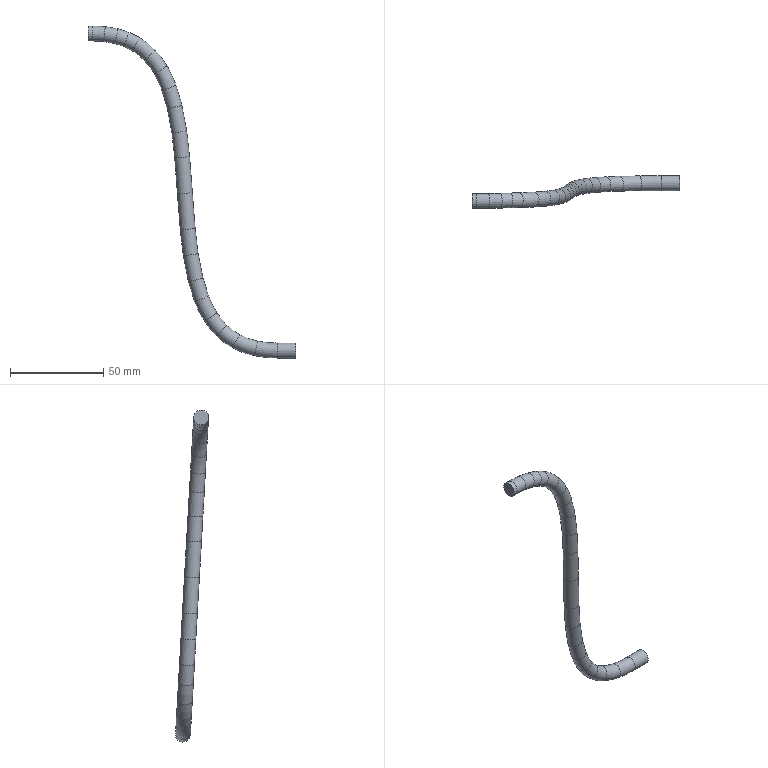Part | STEP file | solid 135 | 1 solid | 24 faces | box 111.404 x 17.72 x 178 mm | volume 11788 mm3 | torus 20 | cylinder 2 | plane 2 | commonest cylinder face diameters 8 x2